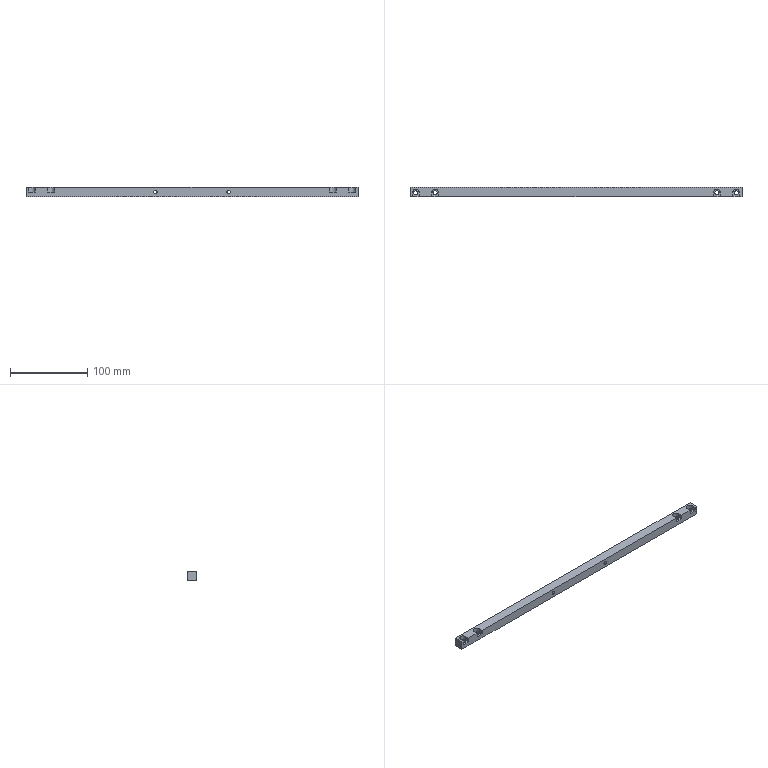Part | SolidWorks | features HoleWzd 2, Extrusion 1, ICE 1 | 1 solid | 40 faces | box 430 x 12 x 12 mm | volume 58809 mm3 | cylinder 20 | plane 20 | commonest cylinder face diameters 5.5 x8 4.5 x4 8 x4 9 x4
STEP:
#1=CARTESIAN_POINT('',(-47.5,1.4,-4.));
#2=VERTEX_POINT('',#1);
#3=CARTESIAN_POINT('',(-47.5,1.4,4.));
#4=VERTEX_POINT('',#3);
#5=CARTESIAN_POINT('',(-47.5,1.4,0.));
#6=DIRECTION('',(0.,1.,0.));
#7=DIRECTION('',(0.,0.,1.));
#8=AXIS2_PLACEMENT_3D('',#5,#6,#7);
#9=CIRCLE('',#8,4.);
#10=EDGE_CURVE('',#2,#4,#9,.T.);
#11=ORIENTED_EDGE('',*,*,#10,.F.);
#12=CARTESIAN_POINT('',(-47.5,6.,-4.));
#13=VERTEX_POINT('',#12);
#14=CARTESIAN_POINT('',(-47.5,6.,-4.));
#15=DIRECTION('',(0.,1.,0.));
#16=VECTOR('',#15,1000.);
#17=LINE('',#14,#16);
#18=EDGE_CURVE('',#2,#13,#17,.T.);
#19=ORIENTED_EDGE('',*,*,#18,.T.);
#20=CARTESIAN_POINT('',(-47.5,6.,4.));
#21=VERTEX_POINT('',#20);
#22=CARTESIAN_POINT('',(-47.5,6.,0.));
#23=DIRECTION('',(0.,1.,0.));
#24=DIRECTION('',(0.,0.,1.));
#25=AXIS2_PLACEMENT_3D('',#22,#23,#24);
#26=CIRCLE('',#25,4.);
#27=EDGE_CURVE('',#13,#21,#26,.T.);
#28=ORIENTED_EDGE('',*,*,#27,.T.);
#29=CARTESIAN_POINT('',(-47.5,6.,4.));
#30=DIRECTION('',(0.,1.,0.));
#31=VECTOR('',#30,1000.);
#32=LINE('',#29,#31);
#33=EDGE_CURVE('',#4,#21,#32,.T.);
#34=ORIENTED_EDGE('',*,*,#33,.F.);
#35=EDGE_LOOP('',(#11,#19,#28,#34));
#36=FACE_OUTER_BOUND('',#35,.T.);
#37=CARTESIAN_POINT('',(-47.5,6.,0.));
#38=DIRECTION('',(0.,1.,0.));
#39=DIRECTION('',(0.,0.,1.));
#40=AXIS2_PLACEMENT_3D('',#37,#38,#39);
#41=CYLINDRICAL_SURFACE('',#40,4.);
#42=ADVANCED_FACE('',(#36),#41,.F.);
#43=CARTESIAN_POINT('',(-47.5,-6.,-2.25));
#44=VERTEX_POINT('',#43);
#45=CARTESIAN_POINT('',(-47.5,-6.,2.25));
#46=VERTEX_POINT('',#45);
#47=CARTESIAN_POINT('',(-47.5,-6.,0.));
#48=DIRECTION('',(0.,1.,0.));
#49=DIRECTION('',(0.,0.,1.));
#50=AXIS2_PLACEMENT_3D('',#47,#48,#49);
#51=CIRCLE('',#50,2.25);
#52=EDGE_CURVE('',#44,#46,#51,.T.);
#53=ORIENTED_EDGE('',*,*,#52,.F.);
#54=CARTESIAN_POINT('',(-47.5,1.4,-2.25));
#55=VERTEX_POINT('',#54);
#56=CARTESIAN_POINT('',(-47.5,6.,-2.25));
#57=DIRECTION('',(0.,1.,0.));
#58=VECTOR('',#57,1000.);
#59=LINE('',#56,#58);
#60=EDGE_CURVE('',#44,#55,#59,.T.);
#61=ORIENTED_EDGE('',*,*,#60,.T.);
#62=CARTESIAN_POINT('',(-47.5,1.4,2.25));
#63=VERTEX_POINT('',#62);
#64=CARTESIAN_POINT('',(-47.5,1.4,0.));
#65=DIRECTION('',(0.,1.,0.));
#66=DIRECTION('',(0.,0.,1.));
#67=AXIS2_PLACEMENT_3D('',#64,#65,#66);
#68=CIRCLE('',#67,2.25);
#69=EDGE_CURVE('',#55,#63,#68,.T.);
#70=ORIENTED_EDGE('',*,*,#69,.T.);
#71=CARTESIAN_POINT('',(-47.5,6.,2.25));
#72=DIRECTION('',(0.,1.,0.));
#73=VECTOR('',#72,1000.);
#74=LINE('',#71,#73);
#75=EDGE_CURVE('',#46,#63,#74,.T.);
#76=ORIENTED_EDGE('',*,*,#75,.F.);
#77=EDGE_LOOP('',(#53,#61,#70,#76));
#78=FACE_OUTER_BOUND('',#77,.T.);
#79=CARTESIAN_POINT('',(-47.5,6.,0.));
#80=DIRECTION('',(0.,1.,0.));
#81=DIRECTION('',(0.,0.,1.));
#82=AXIS2_PLACEMENT_3D('',#79,#80,#81);
#83=CYLINDRICAL_SURFACE('',#82,2.25);
#84=ADVANCED_FACE('',(#78),#83,.F.);
#85=CARTESIAN_POINT('',(47.5,1.4,-4.));
#86=VERTEX_POINT('',#85);
#87=CARTESIAN_POINT('',(47.5,1.4,4.));
#88=VERTEX_POINT('',#87);
#89=CARTESIAN_POINT('',(47.5,1.4,0.));
#90=DIRECTION('',(0.,1.,0.));
#91=DIRECTION('',(0.,0.,1.));
#92=AXIS2_PLACEMENT_3D('',#89,#90,#91);
#93=CIRCLE('',#92,4.);
#94=EDGE_CURVE('',#86,#88,#93,.T.);
#95=ORIENTED_EDGE('',*,*,#94,.F.);
#96=CARTESIAN_POINT('',(47.5,6.,-4.));
#97=VERTEX_POINT('',#96);
#98=CARTESIAN_POINT('',(47.5,6.,-4.));
#99=DIRECTION('',(0.,1.,0.));
#100=VECTOR('',#99,1000.);
#101=LINE('',#98,#100);
#102=EDGE_CURVE('',#86,#97,#101,.T.);
#103=ORIENTED_EDGE('',*,*,#102,.T.);
#104=CARTESIAN_POINT('',(47.5,6.,4.));
#105=VERTEX_POINT('',#104);
#106=CARTESIAN_POINT('',(47.5,6.,0.));
#107=DIRECTION('',(0.,1.,0.));
#108=DIRECTION('',(0.,0.,1.));
#109=AXIS2_PLACEMENT_3D('',#106,#107,#108);
#110=CIRCLE('',#109,4.);
#111=EDGE_CURVE('',#97,#105,#110,.T.);
#112=ORIENTED_EDGE('',*,*,#111,.T.);
#113=CARTESIAN_POINT('',(47.5,6.,4.));
#114=DIRECTION('',(0.,1.,0.));
#115=VECTOR('',#114,1000.);
#116=LINE('',#113,#115);
#117=EDGE_CURVE('',#88,#105,#116,.T.);
#118=ORIENTED_EDGE('',*,*,#117,.F.);
#119=EDGE_LOOP('',(#95,#103,#112,#118));
#120=FACE_OUTER_BOUND('',#119,.T.);
#121=CARTESIAN_POINT('',(47.5,6.,0.));
#122=DIRECTION('',(0.,1.,0.));
#123=DIRECTION('',(0.,0.,1.));
#124=AXIS2_PLACEMENT_3D('',#121,#122,#123);
#125=CYLINDRICAL_SURFACE('',#124,4.);
#126=ADVANCED_FACE('',(#120),#125,.F.);
#127=CARTESIAN_POINT('',(47.5,-6.,-2.25));
#128=VERTEX_POINT('',#127);
#129=CARTESIAN_POINT('',(47.5,-6.,2.25));
#130=VERTEX_POINT('',#129);
#131=CARTESIAN_POINT('',(47.5,-6.,0.));
#132=DIRECTION('',(0.,1.,0.));
#133=DIRECTION('',(0.,0.,1.));
#134=AXIS2_PLACEMENT_3D('',#131,#132,#133);
#135=CIRCLE('',#134,2.25);
#136=EDGE_CURVE('',#128,#130,#135,.T.);
#137=ORIENTED_EDGE('',*,*,#136,.F.);
#138=CARTESIAN_POINT('',(47.5,1.4,-2.25));
#139=VERTEX_POINT('',#138);
#140=CARTESIAN_POINT('',(47.5,6.,-2.25));
#141=DIRECTION('',(0.,1.,0.));
#142=VECTOR('',#141,1000.);
#143=LINE('',#140,#142);
#144=EDGE_CURVE('',#128,#139,#143,.T.);
#145=ORIENTED_EDGE('',*,*,#144,.T.);
#146=CARTESIAN_POINT('',(47.5,1.4,2.25));
#147=VERTEX_POINT('',#146);
#148=CARTESIAN_POINT('',(47.5,1.4,0.));
#149=DIRECTION('',(0.,1.,0.));
#150=DIRECTION('',(0.,0.,1.));
#151=AXIS2_PLACEMENT_3D('',#148,#149,#150);
#152=CIRCLE('',#151,2.25);
#153=EDGE_CURVE('',#139,#147,#152,.T.);
#154=ORIENTED_EDGE('',*,*,#153,.T.);
#155=CARTESIAN_POINT('',(47.5,6.,2.25));
#156=DIRECTION('',(0.,1.,0.));
#157=VECTOR('',#156,1000.);
#158=LINE('',#155,#157);
#159=EDGE_CURVE('',#130,#147,#158,.T.);
#160=ORIENTED_EDGE('',*,*,#159,.F.);
#161=EDGE_LOOP('',(#137,#145,#154,#160));
#162=FACE_OUTER_BOUND('',#161,.T.);
#163=CARTESIAN_POINT('',(47.5,6.,0.));
#164=DIRECTION('',(0.,1.,0.));
#165=DIRECTION('',(0.,0.,1.));
#166=AXIS2_PLACEMENT_3D('',#163,#164,#165);
#167=CYLINDRICAL_SURFACE('',#166,2.25);
#168=ADVANCED_FACE('',(#162),#167,.F.);
#169=CARTESIAN_POINT('',(-210.25,-1.,-6.));
#170=VERTEX_POINT('',#169);
#171=CARTESIAN_POINT('',(-204.75,-1.,-6.));
#172=VERTEX_POINT('',#171);
#173=CARTESIAN_POINT('',(-207.5,-1.,-6.));
#174=DIRECTION('',(0.,0.,1.));
#175=DIRECTION('',(1.,0.,0.));
#176=AXIS2_PLACEMENT_3D('',#173,#174,#175);
#177=CIRCLE('',#176,2.75);
#178=EDGE_CURVE('',#170,#172,#177,.T.);
#179=ORIENTED_EDGE('',*,*,#178,.F.);
#180=CARTESIAN_POINT('',(-210.25,-1.,0.));
#181=VERTEX_POINT('',#180);
#182=CARTESIAN_POINT('',(-210.25,-1.,6.));
#183=DIRECTION('',(0.,0.,1.));
#184=VECTOR('',#183,1000.);
#185=LINE('',#182,#184);
#186=EDGE_CURVE('',#170,#181,#185,.T.);
#187=ORIENTED_EDGE('',*,*,#186,.T.);
#188=CARTESIAN_POINT('',(-204.75,-1.,0.));
#189=VERTEX_POINT('',#188);
#190=CARTESIAN_POINT('',(-207.5,-1.,0.));
#191=DIRECTION('',(0.,0.,-1.));
#192=DIRECTION('',(1.,0.,0.));
#193=AXIS2_PLACEMENT_3D('',#190,#191,#192);
#194=CIRCLE('',#193,2.75);
#195=EDGE_CURVE('',#189,#181,#194,.T.);
#196=ORIENTED_EDGE('',*,*,#195,.F.);
#197=CARTESIAN_POINT('',(-204.75,-1.,6.));
#198=DIRECTION('',(0.,0.,1.));
#199=VECTOR('',#198,1000.);
#200=LINE('',#197,#199);
#201=EDGE_CURVE('',#172,#189,#200,.T.);
#202=ORIENTED_EDGE('',*,*,#201,.F.);
#203=EDGE_LOOP('',(#179,#187,#196,#202));
#204=FACE_OUTER_BOUND('',#203,.T.);
#205=CARTESIAN_POINT('',(-207.5,-1.,6.));
#206=DIRECTION('',(0.,0.,1.));
#207=DIRECTION('',(1.,0.,0.));
#208=AXIS2_PLACEMENT_3D('',#205,#206,#207);
#209=CYLINDRICAL_SURFACE('',#208,2.75);
#210=ADVANCED_FACE('',(#204),#209,.F.);
#211=CARTESIAN_POINT('',(-185.25,-1.,-6.));
#212=VERTEX_POINT('',#211);
#213=CARTESIAN_POINT('',(-179.75,-1.,-6.));
#214=VERTEX_POINT('',#213);
#215=CARTESIAN_POINT('',(-182.5,-1.,-6.));
#216=DIRECTION('',(0.,0.,1.));
#217=DIRECTION('',(1.,0.,0.));
#218=AXIS2_PLACEMENT_3D('',#215,#216,#217);
#219=CIRCLE('',#218,2.75);
#220=EDGE_CURVE('',#212,#214,#219,.T.);
#221=ORIENTED_EDGE('',*,*,#220,.F.);
#222=CARTESIAN_POINT('',(-185.25,-1.,0.));
#223=VERTEX_POINT('',#222);
#224=CARTESIAN_POINT('',(-185.25,-1.,6.));
#225=DIRECTION('',(0.,0.,1.));
#226=VECTOR('',#225,1000.);
#227=LINE('',#224,#226);
#228=EDGE_CURVE('',#212,#223,#227,.T.);
#229=ORIENTED_EDGE('',*,*,#228,.T.);
#230=CARTESIAN_POINT('',(-179.75,-1.,0.));
#231=VERTEX_POINT('',#230);
#232=CARTESIAN_POINT('',(-182.5,-1.,0.));
#233=DIRECTION('',(0.,0.,-1.));
#234=DIRECTION('',(1.,0.,0.));
#235=AXIS2_PLACEMENT_3D('',#232,#233,#234);
#236=CIRCLE('',#235,2.75);
#237=EDGE_CURVE('',#231,#223,#236,.T.);
#238=ORIENTED_EDGE('',*,*,#237,.F.);
#239=CARTESIAN_POINT('',(-179.75,-1.,6.));
#240=DIRECTION('',(0.,0.,1.));
#241=VECTOR('',#240,1000.);
#242=LINE('',#239,#241);
#243=EDGE_CURVE('',#214,#231,#242,.T.);
#244=ORIENTED_EDGE('',*,*,#243,.F.);
#245=EDGE_LOOP('',(#221,#229,#238,#244));
#246=FACE_OUTER_BOUND('',#245,.T.);
#247=CARTESIAN_POINT('',(-182.5,-1.,6.));
#248=DIRECTION('',(0.,0.,1.));
#249=DIRECTION('',(1.,0.,0.));
#250=AXIS2_PLACEMENT_3D('',#247,#248,#249);
#251=CYLINDRICAL_SURFACE('',#250,2.75);
#252=ADVANCED_FACE('',(#246),#251,.F.);
#253=CARTESIAN_POINT('',(179.75,-1.,-6.));
#254=VERTEX_POINT('',#253);
#255=CARTESIAN_POINT('',(185.25,-1.,-6.));
#256=VERTEX_POINT('',#255);
#257=CARTESIAN_POINT('',(182.5,-1.,-6.));
#258=DIRECTION('',(0.,0.,1.));
#259=DIRECTION('',(1.,0.,0.));
#260=AXIS2_PLACEMENT_3D('',#257,#258,#259);
#261=CIRCLE('',#260,2.75);
#262=EDGE_CURVE('',#254,#256,#261,.T.);
#263=ORIENTED_EDGE('',*,*,#262,.F.);
#264=CARTESIAN_POINT('',(179.75,-1.,0.));
#265=VERTEX_POINT('',#264);
#266=CARTESIAN_POINT('',(179.75,-1.,6.));
#267=DIRECTION('',(0.,0.,1.));
#268=VECTOR('',#267,1000.);
#269=LINE('',#266,#268);
#270=EDGE_CURVE('',#254,#265,#269,.T.);
#271=ORIENTED_EDGE('',*,*,#270,.T.);
#272=CARTESIAN_POINT('',(185.25,-1.,0.));
#273=VERTEX_POINT('',#272);
#274=CARTESIAN_POINT('',(182.5,-1.,0.));
#275=DIRECTION('',(0.,0.,-1.));
#276=DIRECTION('',(1.,0.,0.));
#277=AXIS2_PLACEMENT_3D('',#274,#275,#276);
#278=CIRCLE('',#277,2.75);
#279=EDGE_CURVE('',#273,#265,#278,.T.);
#280=ORIENTED_EDGE('',*,*,#279,.F.);
#281=CARTESIAN_POINT('',(185.25,-1.,6.));
#282=DIRECTION('',(0.,0.,1.));
#283=VECTOR('',#282,1000.);
#284=LINE('',#281,#283);
#285=EDGE_CURVE('',#256,#273,#284,.T.);
#286=ORIENTED_EDGE('',*,*,#285,.F.);
#287=EDGE_LOOP('',(#263,#271,#280,#286));
#288=FACE_OUTER_BOUND('',#287,.T.);
#289=CARTESIAN_POINT('',(182.5,-1.,6.));
#290=DIRECTION('',(0.,0.,1.));
#291=DIRECTION('',(1.,0.,0.));
#292=AXIS2_PLACEMENT_3D('',#289,#290,#291);
#293=CYLINDRICAL_SURFACE('',#292,2.75);
#294=ADVANCED_FACE('',(#288),#293,.F.);
#295=CARTESIAN_POINT('',(204.75,-1.,-6.));
#296=VERTEX_POINT('',#295);
#297=CARTESIAN_POINT('',(210.25,-1.,-6.));
#298=VERTEX_POINT('',#297);
#299=CARTESIAN_POINT('',(207.5,-1.,-6.));
#300=DIRECTION('',(0.,0.,1.));
#301=DIRECTION('',(1.,0.,0.));
#302=AXIS2_PLACEMENT_3D('',#299,#300,#301);
#303=CIRCLE('',#302,2.75);
#304=EDGE_CURVE('',#296,#298,#303,.T.);
#305=ORIENTED_EDGE('',*,*,#304,.F.);
#306=CARTESIAN_POINT('',(204.75,-1.,0.));
#307=VERTEX_POINT('',#306);
#308=CARTESIAN_POINT('',(204.75,-1.,6.));
#309=DIRECTION('',(0.,0.,1.));
#310=VECTOR('',#309,1000.);
#311=LINE('',#308,#310);
#312=EDGE_CURVE('',#296,#307,#311,.T.);
#313=ORIENTED_EDGE('',*,*,#312,.T.);
#314=CARTESIAN_POINT('',(210.25,-1.,0.));
#315=VERTEX_POINT('',#314);
#316=CARTESIAN_POINT('',(207.5,-1.,0.));
#317=DIRECTION('',(0.,0.,-1.));
#318=DIRECTION('',(1.,0.,0.));
#319=AXIS2_PLACEMENT_3D('',#316,#317,#318);
#320=CIRCLE('',#319,2.75);
#321=EDGE_CURVE('',#315,#307,#320,.T.);
#322=ORIENTED_EDGE('',*,*,#321,.F.);
#323=CARTESIAN_POINT('',(210.25,-1.,6.));
#324=DIRECTION('',(0.,0.,1.));
#325=VECTOR('',#324,1000.);
#326=LINE('',#323,#325);
#327=EDGE_CURVE('',#298,#315,#326,.T.);
#328=ORIENTED_EDGE('',*,*,#327,.F.);
#329=EDGE_LOOP('',(#305,#313,#322,#328));
#330=FACE_OUTER_BOUND('',#329,.T.);
#331=CARTESIAN_POINT('',(207.5,-1.,6.));
#332=DIRECTION('',(0.,0.,1.));
#333=DIRECTION('',(1.,0.,0.));
#334=AXIS2_PLACEMENT_3D('',#331,#332,#333);
#335=CYLINDRICAL_SURFACE('',#334,2.75);
#336=ADVANCED_FACE('',(#330),#335,.F.);
#337=ORIENTED_EDGE('',*,*,#312,.F.);
#338=CARTESIAN_POINT('',(207.5,-1.,-6.));
#339=DIRECTION('',(0.,0.,1.));
#340=DIRECTION('',(1.,0.,0.));
#341=AXIS2_PLACEMENT_3D('',#338,#339,#340);
#342=CIRCLE('',#341,2.75);
#343=EDGE_CURVE('',#298,#296,#342,.T.);
#344=ORIENTED_EDGE('',*,*,#343,.F.);
#345=ORIENTED_EDGE('',*,*,#327,.T.);
#346=CARTESIAN_POINT('',(207.5,-1.,0.));
#347=DIRECTION('',(0.,0.,-1.));
#348=DIRECTION('',(1.,0.,0.));
#349=AXIS2_PLACEMENT_3D('',#346,#347,#348);
#350=CIRCLE('',#349,2.75);
#351=EDGE_CURVE('',#307,#315,#350,.T.);
#352=ORIENTED_EDGE('',*,*,#351,.F.);
#353=EDGE_LOOP('',(#337,#344,#345,#352));
#354=FACE_OUTER_BOUND('',#353,.T.);
#355=CARTESIAN_POINT('',(207.5,-1.,6.));
#356=DIRECTION('',(0.,0.,1.));
#357=DIRECTION('',(1.,0.,0.));
#358=AXIS2_PLACEMENT_3D('',#355,#356,#357);
#359=CYLINDRICAL_SURFACE('',#358,2.75);
#360=ADVANCED_FACE('',(#354),#359,.F.);
#361=ORIENTED_EDGE('',*,*,#270,.F.);
#362=CARTESIAN_POINT('',(182.5,-1.,-6.));
#363=DIRECTION('',(0.,0.,1.));
#364=DIRECTION('',(1.,0.,0.));
#365=AXIS2_PLACEMENT_3D('',#362,#363,#364);
#366=CIRCLE('',#365,2.75);
#367=EDGE_CURVE('',#256,#254,#366,.T.);
#368=ORIENTED_EDGE('',*,*,#367,.F.);
#369=ORIENTED_EDGE('',*,*,#285,.T.);
#370=CARTESIAN_POINT('',(182.5,-1.,0.));
#371=DIRECTION('',(0.,0.,-1.));
#372=DIRECTION('',(1.,0.,0.));
#373=AXIS2_PLACEMENT_3D('',#370,#371,#372);
#374=CIRCLE('',#373,2.75);
#375=EDGE_CURVE('',#265,#273,#374,.T.);
#376=ORIENTED_EDGE('',*,*,#375,.F.);
#377=EDGE_LOOP('',(#361,#368,#369,#376));
#378=FACE_OUTER_BOUND('',#377,.T.);
#379=CARTESIAN_POINT('',(182.5,-1.,6.));
#380=DIRECTION('',(0.,0.,1.));
#381=DIRECTION('',(1.,0.,0.));
#382=AXIS2_PLACEMENT_3D('',#379,#380,#381);
#383=CYLINDRICAL_SURFACE('',#382,2.75);
#384=ADVANCED_FACE('',(#378),#383,.F.);
#385=ORIENTED_EDGE('',*,*,#228,.F.);
#386=CARTESIAN_POINT('',(-182.5,-1.,-6.));
#387=DIRECTION('',(0.,0.,1.));
#388=DIRECTION('',(1.,0.,0.));
#389=AXIS2_PLACEMENT_3D('',#386,#387,#388);
#390=CIRCLE('',#389,2.75);
#391=EDGE_CURVE('',#214,#212,#390,.T.);
#392=ORIENTED_EDGE('',*,*,#391,.F.);
#393=ORIENTED_EDGE('',*,*,#243,.T.);
#394=CARTESIAN_POINT('',(-182.5,-1.,0.));
#395=DIRECTION('',(0.,0.,-1.));
#396=DIRECTION('',(1.,0.,0.));
#397=AXIS2_PLACEMENT_3D('',#394,#395,#396);
#398=CIRCLE('',#397,2.75);
#399=EDGE_CURVE('',#223,#231,#398,.T.);
#400=ORIENTED_EDGE('',*,*,#399,.F.);
#401=EDGE_LOOP('',(#385,#392,#393,#400));
#402=FACE_OUTER_BOUND('',#401,.T.);
#403=CARTESIAN_POINT('',(-182.5,-1.,6.));
#404=DIRECTION('',(0.,0.,1.));
#405=DIRECTION('',(1.,0.,0.));
#406=AXIS2_PLACEMENT_3D('',#403,#404,#405);
#407=CYLINDRICAL_SURFACE('',#406,2.75);
#408=ADVANCED_FACE('',(#402),#407,.F.);
#409=ORIENTED_EDGE('',*,*,#186,.F.);
#410=CARTESIAN_POINT('',(-207.5,-1.,-6.));
#411=DIRECTION('',(0.,0.,1.));
#412=DIRECTION('',(1.,0.,0.));
#413=AXIS2_PLACEMENT_3D('',#410,#411,#412);
#414=CIRCLE('',#413,2.75);
#415=EDGE_CURVE('',#172,#170,#414,.T.);
#416=ORIENTED_EDGE('',*,*,#415,.F.);
#417=ORIENTED_EDGE('',*,*,#201,.T.);
#418=CARTESIAN_POINT('',(-207.5,-1.,0.));
#419=DIRECTION('',(0.,0.,-1.));
#420=DIRECTION('',(1.,0.,0.));
#421=AXIS2_PLACEMENT_3D('',#418,#419,#420);
#422=CIRCLE('',#421,2.75);
#423=EDGE_CURVE('',#181,#189,#422,.T.);
#424=ORIENTED_EDGE('',*,*,#423,.F.);
#425=EDGE_LOOP('',(#409,#416,#417,#424));
#426=FACE_OUTER_BOUND('',#425,.T.);
#427=CARTESIAN_POINT('',(-207.5,-1.,6.));
#428=DIRECTION('',(0.,0.,1.));
#429=DIRECTION('',(1.,0.,0.));
#430=AXIS2_PLACEMENT_3D('',#427,#428,#429);
#431=CYLINDRICAL_SURFACE('',#430,2.75);
#432=ADVANCED_FACE('',(#426),#431,.F.);
#433=CARTESIAN_POINT('',(215.,-6.,-6.));
#434=VERTEX_POINT('',#433);
#435=CARTESIAN_POINT('',(215.,6.,-6.));
#436=VERTEX_POINT('',#435);
#437=CARTESIAN_POINT('',(215.,6.,-6.));
#438=DIRECTION('',(0.,1.,0.));
#439=VECTOR('',#438,1000.);
#440=LINE('',#437,#439);
#441=EDGE_CURVE('',#434,#436,#440,.T.);
#442=ORIENTED_EDGE('',*,*,#441,.T.);
#443=CARTESIAN_POINT('',(215.,6.,6.));
#444=VERTEX_POINT('',#443);
#445=CARTESIAN_POINT('',(215.,6.,6.));
#446=DIRECTION('',(0.,0.,-1.));
#447=VECTOR('',#446,1000.);
#448=LINE('',#445,#447);
#449=EDGE_CURVE('',#444,#436,#448,.T.);
#450=ORIENTED_EDGE('',*,*,#449,.F.);
#451=CARTESIAN_POINT('',(215.,-6.,6.));
#452=VERTEX_POINT('',#451);
#453=CARTESIAN_POINT('',(215.,6.,6.));
#454=DIRECTION('',(0.,1.,0.));
#455=VECTOR('',#454,1000.);
#456=LINE('',#453,#455);
#457=EDGE_CURVE('',#452,#444,#456,.T.);
#458=ORIENTED_EDGE('',*,*,#457,.F.);
#459=CARTESIAN_POINT('',(215.,-6.,6.));
#460=DIRECTION('',(0.,0.,-1.));
#461=VECTOR('',#460,1000.);
#462=LINE('',#459,#461);
#463=EDGE_CURVE('',#452,#434,#462,.T.);
#464=ORIENTED_EDGE('',*,*,#463,.T.);
#465=EDGE_LOOP('',(#442,#450,#458,#464));
#466=FACE_OUTER_BOUND('',#465,.T.);
#467=CARTESIAN_POINT('',(215.,6.,6.));
#468=DIRECTION('',(-1.,0.,0.));
#469=DIRECTION('',(0.,0.,1.));
#470=AXIS2_PLACEMENT_3D('',#467,#468,#469);
#471=PLANE('',#470);
#472=ADVANCED_FACE('',(#466),#471,.F.);
#473=CARTESIAN_POINT('',(-47.5,6.,0.));
#474=DIRECTION('',(0.,1.,0.));
#475=DIRECTION('',(0.,0.,1.));
#476=AXIS2_PLACEMENT_3D('',#473,#474,#475);
#477=CIRCLE('',#476,4.);
#478=EDGE_CURVE('',#21,#13,#477,.T.);
#479=ORIENTED_EDGE('',*,*,#478,.F.);
#480=ORIENTED_EDGE('',*,*,#27,.F.);
#481=EDGE_LOOP('',(#479,#480));
#482=FACE_BOUND('',#481,.T.);
#483=CARTESIAN_POINT('',(47.5,6.,0.));
#484=DIRECTION('',(0.,1.,0.));
#485=DIRECTION('',(0.,0.,1.));
#486=AXIS2_PLACEMENT_3D('',#483,#484,#485);
#487=CIRCLE('',#486,4.);
#488=EDGE_CURVE('',#105,#97,#487,.T.);
#489=ORIENTED_EDGE('',*,*,#488,.F.);
#490=ORIENTED_EDGE('',*,*,#111,.F.);
#491=EDGE_LOOP('',(#489,#490));
#492=FACE_BOUND('',#491,.T.);
#493=CARTESIAN_POINT('',(-215.,6.,-6.));
#494=VERTEX_POINT('',#493);
#495=CARTESIAN_POINT('',(-215.,6.,-6.));
#496=DIRECTION('',(-1.,0.,0.));
#497=VECTOR('',#496,1000.);
#498=LINE('',#495,#497);
#499=EDGE_CURVE('',#436,#494,#498,.T.);
#500=ORIENTED_EDGE('',*,*,#499,.T.);
#501=CARTESIAN_POINT('',(-215.,6.,6.));
#502=VERTEX_POINT('',#501);
#503=CARTESIAN_POINT('',(-215.,6.,6.));
#504=DIRECTION('',(0.,0.,-1.));
#505=VECTOR('',#504,1000.);
#506=LINE('',#503,#505);
#507=EDGE_CURVE('',#502,#494,#506,.T.);
#508=ORIENTED_EDGE('',*,*,#507,.F.);
#509=CARTESIAN_POINT('',(-215.,6.,6.));
#510=DIRECTION('',(-1.,0.,0.));
#511=VECTOR('',#510,1000.);
#512=LINE('',#509,#511);
#513=EDGE_CURVE('',#444,#502,#512,.T.);
#514=ORIENTED_EDGE('',*,*,#513,.F.);
#515=ORIENTED_EDGE('',*,*,#449,.T.);
#516=EDGE_LOOP('',(#500,#508,#514,#515));
#517=FACE_OUTER_BOUND('',#516,.T.);
#518=CARTESIAN_POINT('',(-215.,6.,6.));
#519=DIRECTION('',(0.,-1.,0.));
#520=DIRECTION('',(0.,0.,-1.));
#521=AXIS2_PLACEMENT_3D('',#518,#519,#520);
#522=PLANE('',#521);
#523=ADVANCED_FACE('',(#482,#492,#517),#522,.F.);
#524=CARTESIAN_POINT('',(-215.,-6.,-6.));
#525=VERTEX_POINT('',#524);
#526=CARTESIAN_POINT('',(-215.,6.,-6.));
#527=DIRECTION('',(0.,-1.,0.));
#528=VECTOR('',#527,1000.);
#529=LINE('',#526,#528);
#530=EDGE_CURVE('',#494,#525,#529,.T.);
#531=ORIENTED_EDGE('',*,*,#530,.T.);
#532=CARTESIAN_POINT('',(-215.,-6.,6.));
#533=VERTEX_POINT('',#532);
#534=CARTESIAN_POINT('',(-215.,-6.,6.));
#535=DIRECTION('',(0.,0.,-1.));
#536=VECTOR('',#535,1000.);
#537=LINE('',#534,#536);
#538=EDGE_CURVE('',#533,#525,#537,.T.);
#539=ORIENTED_EDGE('',*,*,#538,.F.);
#540=CARTESIAN_POINT('',(-215.,6.,6.));
#541=DIRECTION('',(0.,-1.,0.));
#542=VECTOR('',#541,1000.);
#543=LINE('',#540,#542);
#544=EDGE_CURVE('',#502,#533,#543,.T.);
#545=ORIENTED_EDGE('',*,*,#544,.F.);
#546=ORIENTED_EDGE('',*,*,#507,.T.);
#547=EDGE_LOOP('',(#531,#539,#545,#546));
#548=FACE_OUTER_BOUND('',#547,.T.);
#549=CARTESIAN_POINT('',(-215.,6.,6.));
#550=DIRECTION('',(1.,0.,0.));
#551=DIRECTION('',(0.,0.,-1.));
#552=AXIS2_PLACEMENT_3D('',#549,#550,#551);
#553=PLANE('',#552);
#554=ADVANCED_FACE('',(#548),#553,.F.);
#555=CARTESIAN_POINT('',(212.,-6.,6.));
#556=VERTEX_POINT('',#555);
#557=CARTESIAN_POINT('',(-215.,-6.,6.));
#558=DIRECTION('',(1.,0.,0.));
#559=VECTOR('',#558,1000.);
#560=LINE('',#557,#559);
#561=EDGE_CURVE('',#556,#452,#560,.T.);
#562=ORIENTED_EDGE('',*,*,#561,.F.);
#563=CARTESIAN_POINT('',(212.,-6.,0.));
#564=VERTEX_POINT('',#563);
#565=CARTESIAN_POINT('',(212.,-6.,6.));
#566=DIRECTION('',(0.,0.,-1.));
#567=VECTOR('',#566,1000.);
#568=LINE('',#565,#567);
#569=EDGE_CURVE('',#556,#564,#568,.T.);
#570=ORIENTED_EDGE('',*,*,#569,.T.);
#571=CARTESIAN_POINT('',(203.,-6.,0.));
#572=VERTEX_POINT('',#571);
#573=CARTESIAN_POINT('',(-215.,-6.,0.));
#574=DIRECTION('',(1.,0.,0.));
#575=VECTOR('',#574,1000.);
#576=LINE('',#573,#575);
#577=EDGE_CURVE('',#572,#564,#576,.T.);
#578=ORIENTED_EDGE('',*,*,#577,.F.);
#579=CARTESIAN_POINT('',(203.,-6.,6.));
#580=VERTEX_POINT('',#579);
#581=CARTESIAN_POINT('',(203.,-6.,6.));
#582=DIRECTION('',(0.,0.,1.));
#583=VECTOR('',#582,1000.);
#584=LINE('',#581,#583);
#585=EDGE_CURVE('',#572,#580,#584,.T.);
#586=ORIENTED_EDGE('',*,*,#585,.T.);
#587=CARTESIAN_POINT('',(187.,-6.,6.));
#588=VERTEX_POINT('',#587);
#589=CARTESIAN_POINT('',(-215.,-6.,6.));
#590=DIRECTION('',(1.,0.,0.));
#591=VECTOR('',#590,1000.);
#592=LINE('',#589,#591);
#593=EDGE_CURVE('',#588,#580,#592,.T.);
#594=ORIENTED_EDGE('',*,*,#593,.F.);
#595=CARTESIAN_POINT('',(187.,-6.,0.));
#596=VERTEX_POINT('',#595);
#597=CARTESIAN_POINT('',(187.,-6.,6.));
#598=DIRECTION('',(0.,0.,-1.));
#599=VECTOR('',#598,1000.);
#600=LINE('',#597,#599);
#601=EDGE_CURVE('',#588,#596,#600,.T.);
#602=ORIENTED_EDGE('',*,*,#601,.T.);
#603=CARTESIAN_POINT('',(178.,-6.,0.));
#604=VERTEX_POINT('',#603);
#605=CARTESIAN_POINT('',(-215.,-6.,0.));
#606=DIRECTION('',(1.,0.,0.));
#607=VECTOR('',#606,1000.);
#608=LINE('',#605,#607);
#609=EDGE_CURVE('',#604,#596,#608,.T.);
#610=ORIENTED_EDGE('',*,*,#609,.F.);
#611=CARTESIAN_POINT('',(178.,-6.,6.));
#612=VERTEX_POINT('',#611);
#613=CARTESIAN_POINT('',(178.,-6.,6.));
#614=DIRECTION('',(0.,0.,1.));
#615=VECTOR('',#614,1000.);
#616=LINE('',#613,#615);
#617=EDGE_CURVE('',#604,#612,#616,.T.);
#618=ORIENTED_EDGE('',*,*,#617,.T.);
#619=CARTESIAN_POINT('',(-178.,-6.,6.));
#620=VERTEX_POINT('',#619);
#621=CARTESIAN_POINT('',(-215.,-6.,6.));
#622=DIRECTION('',(1.,0.,0.));
#623=VECTOR('',#622,1000.);
#624=LINE('',#621,#623);
#625=EDGE_CURVE('',#620,#612,#624,.T.);
#626=ORIENTED_EDGE('',*,*,#625,.F.);
#627=CARTESIAN_POINT('',(-178.,-6.,0.));
#628=VERTEX_POINT('',#627);
#629=CARTESIAN_POINT('',(-178.,-6.,6.));
#630=DIRECTION('',(0.,0.,-1.));
#631=VECTOR('',#630,1000.);
#632=LINE('',#629,#631);
#633=EDGE_CURVE('',#620,#628,#632,.T.);
#634=ORIENTED_EDGE('',*,*,#633,.T.);
#635=CARTESIAN_POINT('',(-187.,-6.,0.));
#636=VERTEX_POINT('',#635);
#637=CARTESIAN_POINT('',(-215.,-6.,0.));
#638=DIRECTION('',(1.,0.,0.));
#639=VECTOR('',#638,1000.);
#640=LINE('',#637,#639);
#641=EDGE_CURVE('',#636,#628,#640,.T.);
#642=ORIENTED_EDGE('',*,*,#641,.F.);
#643=CARTESIAN_POINT('',(-187.,-6.,6.));
#644=VERTEX_POINT('',#643);
#645=CARTESIAN_POINT('',(-187.,-6.,6.));
#646=DIRECTION('',(0.,0.,1.));
#647=VECTOR('',#646,1000.);
#648=LINE('',#645,#647);
#649=EDGE_CURVE('',#636,#644,#648,.T.);
#650=ORIENTED_EDGE('',*,*,#649,.T.);
#651=CARTESIAN_POINT('',(-203.,-6.,6.));
#652=VERTEX_POINT('',#651);
#653=CARTESIAN_POINT('',(-215.,-6.,6.));
#654=DIRECTION('',(1.,0.,0.));
#655=VECTOR('',#654,1000.);
#656=LINE('',#653,#655);
#657=EDGE_CURVE('',#652,#644,#656,.T.);
#658=ORIENTED_EDGE('',*,*,#657,.F.);
#659=CARTESIAN_POINT('',(-203.,-6.,0.));
#660=VERTEX_POINT('',#659);
#661=CARTESIAN_POINT('',(-203.,-6.,6.));
#662=DIRECTION('',(0.,0.,-1.));
#663=VECTOR('',#662,1000.);
#664=LINE('',#661,#663);
#665=EDGE_CURVE('',#652,#660,#664,.T.);
#666=ORIENTED_EDGE('',*,*,#665,.T.);
#667=CARTESIAN_POINT('',(-212.,-6.,0.));
#668=VERTEX_POINT('',#667);
#669=CARTESIAN_POINT('',(-215.,-6.,0.));
#670=DIRECTION('',(1.,0.,0.));
#671=VECTOR('',#670,1000.);
#672=LINE('',#669,#671);
#673=EDGE_CURVE('',#668,#660,#672,.T.);
#674=ORIENTED_EDGE('',*,*,#673,.F.);
#675=CARTESIAN_POINT('',(-212.,-6.,6.));
#676=VERTEX_POINT('',#675);
#677=CARTESIAN_POINT('',(-212.,-6.,6.));
#678=DIRECTION('',(0.,0.,1.));
#679=VECTOR('',#678,1000.);
#680=LINE('',#677,#679);
#681=EDGE_CURVE('',#668,#676,#680,.T.);
#682=ORIENTED_EDGE('',*,*,#681,.T.);
#683=CARTESIAN_POINT('',(-215.,-6.,6.));
#684=DIRECTION('',(1.,0.,0.));
#685=VECTOR('',#684,1000.);
#686=LINE('',#683,#685);
#687=EDGE_CURVE('',#533,#676,#686,.T.);
#688=ORIENTED_EDGE('',*,*,#687,.F.);
#689=ORIENTED_EDGE('',*,*,#538,.T.);
#690=CARTESIAN_POINT('',(-215.,-6.,-6.));
#691=DIRECTION('',(1.,0.,0.));
#692=VECTOR('',#691,1000.);
#693=LINE('',#690,#692);
#694=EDGE_CURVE('',#525,#434,#693,.T.);
#695=ORIENTED_EDGE('',*,*,#694,.T.);
#696=ORIENTED_EDGE('',*,*,#463,.F.);
#697=EDGE_LOOP('',(#562,#570,#578,#586,#594,#602,#610,#618,#626,#634,#642,#650,#658,#666,#674,#682,#688,#689,#695,#696));
#698=FACE_OUTER_BOUND('',#697,.T.);
#699=CARTESIAN_POINT('',(-47.5,-6.,0.));
#700=DIRECTION('',(0.,1.,0.));
#701=DIRECTION('',(0.,0.,1.));
#702=AXIS2_PLACEMENT_3D('',#699,#700,#701);
#703=CIRCLE('',#702,2.25);
#704=EDGE_CURVE('',#46,#44,#703,.T.);
#705=ORIENTED_EDGE('',*,*,#704,.T.);
#706=ORIENTED_EDGE('',*,*,#52,.T.);
#707=EDGE_LOOP('',(#705,#706));
#708=FACE_BOUND('',#707,.T.);
#709=CARTESIAN_POINT('',(47.5,-6.,0.));
#710=DIRECTION('',(0.,1.,0.));
#711=DIRECTION('',(0.,0.,1.));
#712=AXIS2_PLACEMENT_3D('',#709,#710,#711);
#713=CIRCLE('',#712,2.25);
#714=EDGE_CURVE('',#130,#128,#713,.T.);
#715=ORIENTED_EDGE('',*,*,#714,.T.);
#716=ORIENTED_EDGE('',*,*,#136,.T.);
#717=EDGE_LOOP('',(#715,#716));
#718=FACE_BOUND('',#717,.T.);
#719=CARTESIAN_POINT('',(-215.,-6.,6.));
#720=DIRECTION('',(0.,1.,0.));
#721=DIRECTION('',(0.,0.,1.));
#722=AXIS2_PLACEMENT_3D('',#719,#720,#721);
#723=PLANE('',#722);
#724=ADVANCED_FACE('',(#698,#708,#718),#723,.F.);
#725=CARTESIAN_POINT('',(212.,-1.,6.));
#726=VERTEX_POINT('',#725);
#727=CARTESIAN_POINT('',(212.,-1.,6.));
#728=DIRECTION('',(0.,1.,0.));
#729=VECTOR('',#728,1000.);
#730=LINE('',#727,#729);
#731=EDGE_CURVE('',#556,#726,#730,.T.);
#732=ORIENTED_EDGE('',*,*,#731,.F.);
#733=ORIENTED_EDGE('',*,*,#561,.T.);
#734=ORIENTED_EDGE('',*,*,#457,.T.);
#735=ORIENTED_EDGE('',*,*,#513,.T.);
#736=ORIENTED_EDGE('',*,*,#544,.T.);
#737=ORIENTED_EDGE('',*,*,#687,.T.);
#738=CARTESIAN_POINT('',(-212.,-1.,6.));
#739=VERTEX_POINT('',#738);
#740=CARTESIAN_POINT('',(-212.,-1.,6.));
#741=DIRECTION('',(0.,-1.,0.));
#742=VECTOR('',#741,1000.);
#743=LINE('',#740,#742);
#744=EDGE_CURVE('',#739,#676,#743,.T.);
#745=ORIENTED_EDGE('',*,*,#744,.F.);
#746=CARTESIAN_POINT('',(-203.,-1.,6.));
#747=VERTEX_POINT('',#746);
#748=CARTESIAN_POINT('',(-207.5,-1.,6.));
#749=DIRECTION('',(0.,0.,1.));
#750=DIRECTION('',(1.,0.,0.));
#751=AXIS2_PLACEMENT_3D('',#748,#749,#750);
#752=CIRCLE('',#751,4.5);
#753=EDGE_CURVE('',#747,#739,#752,.T.);
#754=ORIENTED_EDGE('',*,*,#753,.F.);
#755=CARTESIAN_POINT('',(-203.,-1.,6.));
#756=DIRECTION('',(0.,1.,0.));
#757=VECTOR('',#756,1000.);
#758=LINE('',#755,#757);
#759=EDGE_CURVE('',#652,#747,#758,.T.);
#760=ORIENTED_EDGE('',*,*,#759,.F.);
#761=ORIENTED_EDGE('',*,*,#657,.T.);
#762=CARTESIAN_POINT('',(-187.,-1.,6.));
#763=VERTEX_POINT('',#762);
#764=CARTESIAN_POINT('',(-187.,-1.,6.));
#765=DIRECTION('',(0.,-1.,0.));
#766=VECTOR('',#765,1000.);
#767=LINE('',#764,#766);
#768=EDGE_CURVE('',#763,#644,#767,.T.);
#769=ORIENTED_EDGE('',*,*,#768,.F.);
#770=CARTESIAN_POINT('',(-178.,-1.,6.));
#771=VERTEX_POINT('',#770);
#772=CARTESIAN_POINT('',(-182.5,-1.,6.));
#773=DIRECTION('',(0.,0.,1.));
#774=DIRECTION('',(1.,0.,0.));
#775=AXIS2_PLACEMENT_3D('',#772,#773,#774);
#776=CIRCLE('',#775,4.5);
#777=EDGE_CURVE('',#771,#763,#776,.T.);
#778=ORIENTED_EDGE('',*,*,#777,.F.);
#779=CARTESIAN_POINT('',(-178.,-1.,6.));
#780=DIRECTION('',(0.,1.,0.));
#781=VECTOR('',#780,1000.);
#782=LINE('',#779,#781);
#783=EDGE_CURVE('',#620,#771,#782,.T.);
#784=ORIENTED_EDGE('',*,*,#783,.F.);
#785=ORIENTED_EDGE('',*,*,#625,.T.);
#786=CARTESIAN_POINT('',(178.,-1.,6.));
#787=VERTEX_POINT('',#786);
#788=CARTESIAN_POINT('',(178.,-1.,6.));
#789=DIRECTION('',(0.,-1.,0.));
#790=VECTOR('',#789,1000.);
#791=LINE('',#788,#790);
#792=EDGE_CURVE('',#787,#612,#791,.T.);
#793=ORIENTED_EDGE('',*,*,#792,.F.);
#794=CARTESIAN_POINT('',(187.,-1.,6.));
#795=VERTEX_POINT('',#794);
#796=CARTESIAN_POINT('',(182.5,-1.,6.));
#797=DIRECTION('',(0.,0.,1.));
#798=DIRECTION('',(1.,0.,0.));
#799=AXIS2_PLACEMENT_3D('',#796,#797,#798);
#800=CIRCLE('',#799,4.5);
#801=EDGE_CURVE('',#795,#787,#800,.T.);
#802=ORIENTED_EDGE('',*,*,#801,.F.);
#803=CARTESIAN_POINT('',(187.,-1.,6.));
#804=DIRECTION('',(0.,1.,0.));
#805=VECTOR('',#804,1000.);
#806=LINE('',#803,#805);
#807=EDGE_CURVE('',#588,#795,#806,.T.);
#808=ORIENTED_EDGE('',*,*,#807,.F.);
#809=ORIENTED_EDGE('',*,*,#593,.T.);
#810=CARTESIAN_POINT('',(203.,-1.,6.));
#811=VERTEX_POINT('',#810);
#812=CARTESIAN_POINT('',(203.,-1.,6.));
#813=DIRECTION('',(0.,-1.,0.));
#814=VECTOR('',#813,1000.);
#815=LINE('',#812,#814);
#816=EDGE_CURVE('',#811,#580,#815,.T.);
#817=ORIENTED_EDGE('',*,*,#816,.F.);
#818=CARTESIAN_POINT('',(207.5,-1.,6.));
#819=DIRECTION('',(0.,0.,1.));
#820=DIRECTION('',(1.,0.,0.));
#821=AXIS2_PLACEMENT_3D('',#818,#819,#820);
#822=CIRCLE('',#821,4.5);
#823=EDGE_CURVE('',#726,#811,#822,.T.);
#824=ORIENTED_EDGE('',*,*,#823,.F.);
#825=EDGE_LOOP('',(#732,#733,#734,#735,#736,#737,#745,#754,#760,#761,#769,#778,#784,#785,#793,#802,#808,#809,#817,#824));
#826=FACE_OUTER_BOUND('',#825,.T.);
#827=CARTESIAN_POINT('',(0.,0.,6.));
#828=DIRECTION('',(0.,0.,1.));
#829=DIRECTION('',(1.,0.,0.));
#830=AXIS2_PLACEMENT_3D('',#827,#828,#829);
#831=PLANE('',#830);
#832=ADVANCED_FACE('',(#826),#831,.T.);
#833=ORIENTED_EDGE('',*,*,#415,.T.);
#834=ORIENTED_EDGE('',*,*,#178,.T.);
#835=EDGE_LOOP('',(#833,#834));
#836=FACE_BOUND('',#835,.T.);
#837=ORIENTED_EDGE('',*,*,#391,.T.);
#838=ORIENTED_EDGE('',*,*,#220,.T.);
#839=EDGE_LOOP('',(#837,#838));
#840=FACE_BOUND('',#839,.T.);
#841=ORIENTED_EDGE('',*,*,#367,.T.);
#842=ORIENTED_EDGE('',*,*,#262,.T.);
#843=EDGE_LOOP('',(#841,#842));
#844=FACE_BOUND('',#843,.T.);
#845=ORIENTED_EDGE('',*,*,#343,.T.);
#846=ORIENTED_EDGE('',*,*,#304,.T.);
#847=EDGE_LOOP('',(#845,#846));
#848=FACE_BOUND('',#847,.T.);
#849=ORIENTED_EDGE('',*,*,#441,.F.);
#850=ORIENTED_EDGE('',*,*,#694,.F.);
#851=ORIENTED_EDGE('',*,*,#530,.F.);
#852=ORIENTED_EDGE('',*,*,#499,.F.);
#853=EDGE_LOOP('',(#849,#850,#851,#852));
#854=FACE_OUTER_BOUND('',#853,.T.);
#855=CARTESIAN_POINT('',(0.,0.,-6.));
#856=DIRECTION('',(0.,0.,1.));
#857=DIRECTION('',(1.,0.,0.));
#858=AXIS2_PLACEMENT_3D('',#855,#856,#857);
#859=PLANE('',#858);
#860=ADVANCED_FACE('',(#836,#840,#844,#848,#854),#859,.F.);
#861=ORIENTED_EDGE('',*,*,#144,.F.);
#862=ORIENTED_EDGE('',*,*,#714,.F.);
#863=ORIENTED_EDGE('',*,*,#159,.T.);
#864=CARTESIAN_POINT('',(47.5,1.4,0.));
#865=DIRECTION('',(0.,1.,0.));
#866=DIRECTION('',(0.,0.,1.));
#867=AXIS2_PLACEMENT_3D('',#864,#865,#866);
#868=CIRCLE('',#867,2.25);
#869=EDGE_CURVE('',#147,#139,#868,.T.);
#870=ORIENTED_EDGE('',*,*,#869,.T.);
#871=EDGE_LOOP('',(#861,#862,#863,#870));
#872=FACE_OUTER_BOUND('',#871,.T.);
#873=CARTESIAN_POINT('',(47.5,6.,0.));
#874=DIRECTION('',(0.,1.,0.));
#875=DIRECTION('',(0.,0.,1.));
#876=AXIS2_PLACEMENT_3D('',#873,#874,#875);
#877=CYLINDRICAL_SURFACE('',#876,2.25);
#878=ADVANCED_FACE('',(#872),#877,.F.);
#879=ORIENTED_EDGE('',*,*,#869,.F.);
#880=ORIENTED_EDGE('',*,*,#153,.F.);
#881=EDGE_LOOP('',(#879,#880));
#882=FACE_BOUND('',#881,.T.);
#883=CARTESIAN_POINT('',(47.5,1.4,0.));
#884=DIRECTION('',(0.,1.,0.));
#885=DIRECTION('',(0.,0.,1.));
#886=AXIS2_PLACEMENT_3D('',#883,#884,#885);
#887=CIRCLE('',#886,4.);
#888=EDGE_CURVE('',#88,#86,#887,.T.);
#889=ORIENTED_EDGE('',*,*,#888,.T.);
#890=ORIENTED_EDGE('',*,*,#94,.T.);
#891=EDGE_LOOP('',(#889,#890));
#892=FACE_OUTER_BOUND('',#891,.T.);
#893=CARTESIAN_POINT('',(49.75,1.4,0.));
#894=DIRECTION('',(0.,-1.,0.));
#895=DIRECTION('',(0.,0.,-1.));
#896=AXIS2_PLACEMENT_3D('',#893,#894,#895);
#897=PLANE('',#896);
#898=ADVANCED_FACE('',(#882,#892),#897,.F.);
#899=ORIENTED_EDGE('',*,*,#102,.F.);
#900=ORIENTED_EDGE('',*,*,#888,.F.);
#901=ORIENTED_EDGE('',*,*,#117,.T.);
#902=ORIENTED_EDGE('',*,*,#488,.T.);
#903=EDGE_LOOP('',(#899,#900,#901,#902));
#904=FACE_OUTER_BOUND('',#903,.T.);
#905=CARTESIAN_POINT('',(47.5,6.,0.));
#906=DIRECTION('',(0.,1.,0.));
#907=DIRECTION('',(0.,0.,1.));
#908=AXIS2_PLACEMENT_3D('',#905,#906,#907);
#909=CYLINDRICAL_SURFACE('',#908,4.);
#910=ADVANCED_FACE('',(#904),#909,.F.);
#911=ORIENTED_EDGE('',*,*,#60,.F.);
#912=ORIENTED_EDGE('',*,*,#704,.F.);
#913=ORIENTED_EDGE('',*,*,#75,.T.);
#914=CARTESIAN_POINT('',(-47.5,1.4,0.));
#915=DIRECTION('',(0.,1.,0.));
#916=DIRECTION('',(0.,0.,1.));
#917=AXIS2_PLACEMENT_3D('',#914,#915,#916);
#918=CIRCLE('',#917,2.25);
#919=EDGE_CURVE('',#63,#55,#918,.T.);
#920=ORIENTED_EDGE('',*,*,#919,.T.);
#921=EDGE_LOOP('',(#911,#912,#913,#920));
#922=FACE_OUTER_BOUND('',#921,.T.);
#923=CARTESIAN_POINT('',(-47.5,6.,0.));
#924=DIRECTION('',(0.,1.,0.));
#925=DIRECTION('',(0.,0.,1.));
#926=AXIS2_PLACEMENT_3D('',#923,#924,#925);
#927=CYLINDRICAL_SURFACE('',#926,2.25);
#928=ADVANCED_FACE('',(#922),#927,.F.);
#929=ORIENTED_EDGE('',*,*,#919,.F.);
#930=ORIENTED_EDGE('',*,*,#69,.F.);
#931=EDGE_LOOP('',(#929,#930));
#932=FACE_BOUND('',#931,.T.);
#933=CARTESIAN_POINT('',(-47.5,1.4,0.));
#934=DIRECTION('',(0.,1.,0.));
#935=DIRECTION('',(0.,0.,1.));
#936=AXIS2_PLACEMENT_3D('',#933,#934,#935);
#937=CIRCLE('',#936,4.);
#938=EDGE_CURVE('',#4,#2,#937,.T.);
#939=ORIENTED_EDGE('',*,*,#938,.T.);
#940=ORIENTED_EDGE('',*,*,#10,.T.);
#941=EDGE_LOOP('',(#939,#940));
#942=FACE_OUTER_BOUND('',#941,.T.);
#943=CARTESIAN_POINT('',(-45.25,1.4,0.));
#944=DIRECTION('',(0.,-1.,0.));
#945=DIRECTION('',(0.,0.,-1.));
#946=AXIS2_PLACEMENT_3D('',#943,#944,#945);
#947=PLANE('',#946);
#948=ADVANCED_FACE('',(#932,#942),#947,.F.);
#949=ORIENTED_EDGE('',*,*,#18,.F.);
#950=ORIENTED_EDGE('',*,*,#938,.F.);
#951=ORIENTED_EDGE('',*,*,#33,.T.);
#952=ORIENTED_EDGE('',*,*,#478,.T.);
#953=EDGE_LOOP('',(#949,#950,#951,#952));
#954=FACE_OUTER_BOUND('',#953,.T.);
#955=CARTESIAN_POINT('',(-47.5,6.,0.));
#956=DIRECTION('',(0.,1.,0.));
#957=DIRECTION('',(0.,0.,1.));
#958=AXIS2_PLACEMENT_3D('',#955,#956,#957);
#959=CYLINDRICAL_SURFACE('',#958,4.);
#960=ADVANCED_FACE('',(#954),#959,.F.);
#961=ORIENTED_EDGE('',*,*,#759,.T.);
#962=CARTESIAN_POINT('',(-203.,-1.,0.));
#963=VERTEX_POINT('',#962);
#964=CARTESIAN_POINT('',(-203.,-1.,0.));
#965=DIRECTION('',(0.,0.,1.));
#966=VECTOR('',#965,1000.);
#967=LINE('',#964,#966);
#968=EDGE_CURVE('',#963,#747,#967,.T.);
#969=ORIENTED_EDGE('',*,*,#968,.F.);
#970=CARTESIAN_POINT('',(-203.,-1.,0.));
#971=DIRECTION('',(0.,1.,0.));
#972=VECTOR('',#971,1000.);
#973=LINE('',#970,#972);
#974=EDGE_CURVE('',#660,#963,#973,.T.);
#975=ORIENTED_EDGE('',*,*,#974,.F.);
#976=ORIENTED_EDGE('',*,*,#665,.F.);
#977=EDGE_LOOP('',(#961,#969,#975,#976));
#978=FACE_OUTER_BOUND('',#977,.T.);
#979=CARTESIAN_POINT('',(-203.,-1.,0.));
#980=DIRECTION('',(1.,0.,0.));
#981=DIRECTION('',(0.,1.,0.));
#982=AXIS2_PLACEMENT_3D('',#979,#980,#981);
#983=PLANE('',#982);
#984=ADVANCED_FACE('',(#978),#983,.F.);
#985=CARTESIAN_POINT('',(-212.,-1.,0.));
#986=VERTEX_POINT('',#985);
#987=CARTESIAN_POINT('',(-212.,-1.,0.));
#988=DIRECTION('',(0.,-1.,0.));
#989=VECTOR('',#988,1000.);
#990=LINE('',#987,#989);
#991=EDGE_CURVE('',#986,#668,#990,.T.);
#992=ORIENTED_EDGE('',*,*,#991,.F.);
#993=CARTESIAN_POINT('',(-212.,-1.,0.));
#994=DIRECTION('',(0.,0.,1.));
#995=VECTOR('',#994,1000.);
#996=LINE('',#993,#995);
#997=EDGE_CURVE('',#986,#739,#996,.T.);
#998=ORIENTED_EDGE('',*,*,#997,.T.);
#999=ORIENTED_EDGE('',*,*,#744,.T.);
#1000=ORIENTED_EDGE('',*,*,#681,.F.);
#1001=EDGE_LOOP('',(#992,#998,#999,#1000));
#1002=FACE_OUTER_BOUND('',#1001,.T.);
#1003=CARTESIAN_POINT('',(-212.,-1.,0.));
#1004=DIRECTION('',(-1.,0.,0.));
#1005=DIRECTION('',(0.,-1.,0.));
#1006=AXIS2_PLACEMENT_3D('',#1003,#1004,#1005);
#1007=PLANE('',#1006);
#1008=ADVANCED_FACE('',(#1002),#1007,.F.);
#1009=ORIENTED_EDGE('',*,*,#195,.T.);
#1010=ORIENTED_EDGE('',*,*,#423,.T.);
#1011=EDGE_LOOP('',(#1009,#1010));
#1012=FACE_BOUND('',#1011,.T.);
#1013=ORIENTED_EDGE('',*,*,#673,.T.);
#1014=ORIENTED_EDGE('',*,*,#974,.T.);
#1015=CARTESIAN_POINT('',(-207.5,-1.,0.));
#1016=DIRECTION('',(0.,0.,1.));
#1017=DIRECTION('',(1.,0.,0.));
#1018=AXIS2_PLACEMENT_3D('',#1015,#1016,#1017);
#1019=CIRCLE('',#1018,4.5);
#1020=EDGE_CURVE('',#963,#986,#1019,.T.);
#1021=ORIENTED_EDGE('',*,*,#1020,.T.);
#1022=ORIENTED_EDGE('',*,*,#991,.T.);
#1023=EDGE_LOOP('',(#1013,#1014,#1021,#1022));
#1024=FACE_OUTER_BOUND('',#1023,.T.);
#1025=CARTESIAN_POINT('',(-207.5,-1.,0.));
#1026=DIRECTION('',(0.,0.,1.));
#1027=DIRECTION('',(1.,0.,0.));
#1028=AXIS2_PLACEMENT_3D('',#1025,#1026,#1027);
#1029=PLANE('',#1028);
#1030=ADVANCED_FACE('',(#1012,#1024),#1029,.T.);
#1031=ORIENTED_EDGE('',*,*,#753,.T.);
#1032=ORIENTED_EDGE('',*,*,#997,.F.);
#1033=ORIENTED_EDGE('',*,*,#1020,.F.);
#1034=ORIENTED_EDGE('',*,*,#968,.T.);
#1035=EDGE_LOOP('',(#1031,#1032,#1033,#1034));
#1036=FACE_OUTER_BOUND('',#1035,.T.);
#1037=CARTESIAN_POINT('',(-207.5,-1.,0.));
#1038=DIRECTION('',(0.,0.,1.));
#1039=DIRECTION('',(1.,0.,0.));
#1040=AXIS2_PLACEMENT_3D('',#1037,#1038,#1039);
#1041=CYLINDRICAL_SURFACE('',#1040,4.5);
#1042=ADVANCED_FACE('',(#1036),#1041,.F.);
#1043=ORIENTED_EDGE('',*,*,#783,.T.);
#1044=CARTESIAN_POINT('',(-178.,-1.,0.));
#1045=VERTEX_POINT('',#1044);
#1046=CARTESIAN_POINT('',(-178.,-1.,0.));
#1047=DIRECTION('',(0.,0.,1.));
#1048=VECTOR('',#1047,1000.);
#1049=LINE('',#1046,#1048);
#1050=EDGE_CURVE('',#1045,#771,#1049,.T.);
#1051=ORIENTED_EDGE('',*,*,#1050,.F.);
#1052=CARTESIAN_POINT('',(-178.,-1.,0.));
#1053=DIRECTION('',(0.,1.,0.));
#1054=VECTOR('',#1053,1000.);
#1055=LINE('',#1052,#1054);
#1056=EDGE_CURVE('',#628,#1045,#1055,.T.);
#1057=ORIENTED_EDGE('',*,*,#1056,.F.);
#1058=ORIENTED_EDGE('',*,*,#633,.F.);
#1059=EDGE_LOOP('',(#1043,#1051,#1057,#1058));
#1060=FACE_OUTER_BOUND('',#1059,.T.);
#1061=CARTESIAN_POINT('',(-178.,-1.,0.));
#1062=DIRECTION('',(1.,0.,0.));
#1063=DIRECTION('',(0.,1.,0.));
#1064=AXIS2_PLACEMENT_3D('',#1061,#1062,#1063);
#1065=PLANE('',#1064);
#1066=ADVANCED_FACE('',(#1060),#1065,.F.);
#1067=CARTESIAN_POINT('',(-187.,-1.,0.));
#1068=VERTEX_POINT('',#1067);
#1069=CARTESIAN_POINT('',(-187.,-1.,0.));
#1070=DIRECTION('',(0.,-1.,0.));
#1071=VECTOR('',#1070,1000.);
#1072=LINE('',#1069,#1071);
#1073=EDGE_CURVE('',#1068,#636,#1072,.T.);
#1074=ORIENTED_EDGE('',*,*,#1073,.F.);
#1075=CARTESIAN_POINT('',(-187.,-1.,0.));
#1076=DIRECTION('',(0.,0.,1.));
#1077=VECTOR('',#1076,1000.);
#1078=LINE('',#1075,#1077);
#1079=EDGE_CURVE('',#1068,#763,#1078,.T.);
#1080=ORIENTED_EDGE('',*,*,#1079,.T.);
#1081=ORIENTED_EDGE('',*,*,#768,.T.);
#1082=ORIENTED_EDGE('',*,*,#649,.F.);
#1083=EDGE_LOOP('',(#1074,#1080,#1081,#1082));
#1084=FACE_OUTER_BOUND('',#1083,.T.);
#1085=CARTESIAN_POINT('',(-187.,-1.,0.));
#1086=DIRECTION('',(-1.,0.,0.));
#1087=DIRECTION('',(0.,-1.,0.));
#1088=AXIS2_PLACEMENT_3D('',#1085,#1086,#1087);
#1089=PLANE('',#1088);
#1090=ADVANCED_FACE('',(#1084),#1089,.F.);
#1091=ORIENTED_EDGE('',*,*,#237,.T.);
#1092=ORIENTED_EDGE('',*,*,#399,.T.);
#1093=EDGE_LOOP('',(#1091,#1092));
#1094=FACE_BOUND('',#1093,.T.);
#1095=ORIENTED_EDGE('',*,*,#641,.T.);
#1096=ORIENTED_EDGE('',*,*,#1056,.T.);
#1097=CARTESIAN_POINT('',(-182.5,-1.,0.));
#1098=DIRECTION('',(0.,0.,1.));
#1099=DIRECTION('',(1.,0.,0.));
#1100=AXIS2_PLACEMENT_3D('',#1097,#1098,#1099);
#1101=CIRCLE('',#1100,4.5);
#1102=EDGE_CURVE('',#1045,#1068,#1101,.T.);
#1103=ORIENTED_EDGE('',*,*,#1102,.T.);
#1104=ORIENTED_EDGE('',*,*,#1073,.T.);
#1105=EDGE_LOOP('',(#1095,#1096,#1103,#1104));
#1106=FACE_OUTER_BOUND('',#1105,.T.);
#1107=CARTESIAN_POINT('',(-182.5,-1.,0.));
#1108=DIRECTION('',(0.,0.,1.));
#1109=DIRECTION('',(1.,0.,0.));
#1110=AXIS2_PLACEMENT_3D('',#1107,#1108,#1109);
#1111=PLANE('',#1110);
#1112=ADVANCED_FACE('',(#1094,#1106),#1111,.T.);
#1113=ORIENTED_EDGE('',*,*,#777,.T.);
#1114=ORIENTED_EDGE('',*,*,#1079,.F.);
#1115=ORIENTED_EDGE('',*,*,#1102,.F.);
#1116=ORIENTED_EDGE('',*,*,#1050,.T.);
#1117=EDGE_LOOP('',(#1113,#1114,#1115,#1116));
#1118=FACE_OUTER_BOUND('',#1117,.T.);
#1119=CARTESIAN_POINT('',(-182.5,-1.,0.));
#1120=DIRECTION('',(0.,0.,1.));
#1121=DIRECTION('',(1.,0.,0.));
#1122=AXIS2_PLACEMENT_3D('',#1119,#1120,#1121);
#1123=CYLINDRICAL_SURFACE('',#1122,4.5);
#1124=ADVANCED_FACE('',(#1118),#1123,.F.);
#1125=ORIENTED_EDGE('',*,*,#807,.T.);
#1126=CARTESIAN_POINT('',(187.,-1.,0.));
#1127=VERTEX_POINT('',#1126);
#1128=CARTESIAN_POINT('',(187.,-1.,0.));
#1129=DIRECTION('',(0.,0.,1.));
#1130=VECTOR('',#1129,1000.);
#1131=LINE('',#1128,#1130);
#1132=EDGE_CURVE('',#1127,#795,#1131,.T.);
#1133=ORIENTED_EDGE('',*,*,#1132,.F.);
#1134=CARTESIAN_POINT('',(187.,-1.,0.));
#1135=DIRECTION('',(0.,1.,0.));
#1136=VECTOR('',#1135,1000.);
#1137=LINE('',#1134,#1136);
#1138=EDGE_CURVE('',#596,#1127,#1137,.T.);
#1139=ORIENTED_EDGE('',*,*,#1138,.F.);
#1140=ORIENTED_EDGE('',*,*,#601,.F.);
#1141=EDGE_LOOP('',(#1125,#1133,#1139,#1140));
#1142=FACE_OUTER_BOUND('',#1141,.T.);
#1143=CARTESIAN_POINT('',(187.,-1.,0.));
#1144=DIRECTION('',(1.,0.,0.));
#1145=DIRECTION('',(0.,1.,0.));
#1146=AXIS2_PLACEMENT_3D('',#1143,#1144,#1145);
#1147=PLANE('',#1146);
#1148=ADVANCED_FACE('',(#1142),#1147,.F.);
#1149=CARTESIAN_POINT('',(178.,-1.,0.));
#1150=VERTEX_POINT('',#1149);
#1151=CARTESIAN_POINT('',(178.,-1.,0.));
#1152=DIRECTION('',(0.,-1.,0.));
#1153=VECTOR('',#1152,1000.);
#1154=LINE('',#1151,#1153);
#1155=EDGE_CURVE('',#1150,#604,#1154,.T.);
#1156=ORIENTED_EDGE('',*,*,#1155,.F.);
#1157=CARTESIAN_POINT('',(178.,-1.,0.));
#1158=DIRECTION('',(0.,0.,1.));
#1159=VECTOR('',#1158,1000.);
#1160=LINE('',#1157,#1159);
#1161=EDGE_CURVE('',#1150,#787,#1160,.T.);
#1162=ORIENTED_EDGE('',*,*,#1161,.T.);
#1163=ORIENTED_EDGE('',*,*,#792,.T.);
#1164=ORIENTED_EDGE('',*,*,#617,.F.);
#1165=EDGE_LOOP('',(#1156,#1162,#1163,#1164));
#1166=FACE_OUTER_BOUND('',#1165,.T.);
#1167=CARTESIAN_POINT('',(178.,-1.,0.));
#1168=DIRECTION('',(-1.,0.,0.));
#1169=DIRECTION('',(0.,-1.,0.));
#1170=AXIS2_PLACEMENT_3D('',#1167,#1168,#1169);
#1171=PLANE('',#1170);
#1172=ADVANCED_FACE('',(#1166),#1171,.F.);
#1173=ORIENTED_EDGE('',*,*,#279,.T.);
#1174=ORIENTED_EDGE('',*,*,#375,.T.);
#1175=EDGE_LOOP('',(#1173,#1174));
#1176=FACE_BOUND('',#1175,.T.);
#1177=ORIENTED_EDGE('',*,*,#609,.T.);
#1178=ORIENTED_EDGE('',*,*,#1138,.T.);
#1179=CARTESIAN_POINT('',(182.5,-1.,0.));
#1180=DIRECTION('',(0.,0.,1.));
#1181=DIRECTION('',(1.,0.,0.));
#1182=AXIS2_PLACEMENT_3D('',#1179,#1180,#1181);
#1183=CIRCLE('',#1182,4.5);
#1184=EDGE_CURVE('',#1127,#1150,#1183,.T.);
#1185=ORIENTED_EDGE('',*,*,#1184,.T.);
#1186=ORIENTED_EDGE('',*,*,#1155,.T.);
#1187=EDGE_LOOP('',(#1177,#1178,#1185,#1186));
#1188=FACE_OUTER_BOUND('',#1187,.T.);
#1189=CARTESIAN_POINT('',(182.5,-1.,0.));
#1190=DIRECTION('',(0.,0.,1.));
#1191=DIRECTION('',(1.,0.,0.));
#1192=AXIS2_PLACEMENT_3D('',#1189,#1190,#1191);
#1193=PLANE('',#1192);
#1194=ADVANCED_FACE('',(#1176,#1188),#1193,.T.);
#1195=ORIENTED_EDGE('',*,*,#801,.T.);
#1196=ORIENTED_EDGE('',*,*,#1161,.F.);
#1197=ORIENTED_EDGE('',*,*,#1184,.F.);
#1198=ORIENTED_EDGE('',*,*,#1132,.T.);
#1199=EDGE_LOOP('',(#1195,#1196,#1197,#1198));
#1200=FACE_OUTER_BOUND('',#1199,.T.);
#1201=CARTESIAN_POINT('',(182.5,-1.,0.));
#1202=DIRECTION('',(0.,0.,1.));
#1203=DIRECTION('',(1.,0.,0.));
#1204=AXIS2_PLACEMENT_3D('',#1201,#1202,#1203);
#1205=CYLINDRICAL_SURFACE('',#1204,4.5);
#1206=ADVANCED_FACE('',(#1200),#1205,.F.);
#1207=ORIENTED_EDGE('',*,*,#731,.T.);
#1208=CARTESIAN_POINT('',(212.,-1.,0.));
#1209=VERTEX_POINT('',#1208);
#1210=CARTESIAN_POINT('',(212.,-1.,0.));
#1211=DIRECTION('',(0.,0.,1.));
#1212=VECTOR('',#1211,1000.);
#1213=LINE('',#1210,#1212);
#1214=EDGE_CURVE('',#1209,#726,#1213,.T.);
#1215=ORIENTED_EDGE('',*,*,#1214,.F.);
#1216=CARTESIAN_POINT('',(212.,-1.,0.));
#1217=DIRECTION('',(0.,1.,0.));
#1218=VECTOR('',#1217,1000.);
#1219=LINE('',#1216,#1218);
#1220=EDGE_CURVE('',#564,#1209,#1219,.T.);
#1221=ORIENTED_EDGE('',*,*,#1220,.F.);
#1222=ORIENTED_EDGE('',*,*,#569,.F.);
#1223=EDGE_LOOP('',(#1207,#1215,#1221,#1222));
#1224=FACE_OUTER_BOUND('',#1223,.T.);
#1225=CARTESIAN_POINT('',(212.,-1.,0.));
#1226=DIRECTION('',(1.,0.,0.));
#1227=DIRECTION('',(0.,1.,0.));
#1228=AXIS2_PLACEMENT_3D('',#1225,#1226,#1227);
#1229=PLANE('',#1228);
#1230=ADVANCED_FACE('',(#1224),#1229,.F.);
#1231=CARTESIAN_POINT('',(203.,-1.,0.));
#1232=VERTEX_POINT('',#1231);
#1233=CARTESIAN_POINT('',(203.,-1.,0.));
#1234=DIRECTION('',(0.,-1.,0.));
#1235=VECTOR('',#1234,1000.);
#1236=LINE('',#1233,#1235);
#1237=EDGE_CURVE('',#1232,#572,#1236,.T.);
#1238=ORIENTED_EDGE('',*,*,#1237,.F.);
#1239=CARTESIAN_POINT('',(203.,-1.,0.));
#1240=DIRECTION('',(0.,0.,1.));
#1241=VECTOR('',#1240,1000.);
#1242=LINE('',#1239,#1241);
#1243=EDGE_CURVE('',#1232,#811,#1242,.T.);
#1244=ORIENTED_EDGE('',*,*,#1243,.T.);
#1245=ORIENTED_EDGE('',*,*,#816,.T.);
#1246=ORIENTED_EDGE('',*,*,#585,.F.);
#1247=EDGE_LOOP('',(#1238,#1244,#1245,#1246));
#1248=FACE_OUTER_BOUND('',#1247,.T.);
#1249=CARTESIAN_POINT('',(203.,-1.,0.));
#1250=DIRECTION('',(-1.,0.,0.));
#1251=DIRECTION('',(0.,-1.,0.));
#1252=AXIS2_PLACEMENT_3D('',#1249,#1250,#1251);
#1253=PLANE('',#1252);
#1254=ADVANCED_FACE('',(#1248),#1253,.F.);
#1255=ORIENTED_EDGE('',*,*,#321,.T.);
#1256=ORIENTED_EDGE('',*,*,#351,.T.);
#1257=EDGE_LOOP('',(#1255,#1256));
#1258=FACE_BOUND('',#1257,.T.);
#1259=ORIENTED_EDGE('',*,*,#577,.T.);
#1260=ORIENTED_EDGE('',*,*,#1220,.T.);
#1261=CARTESIAN_POINT('',(207.5,-1.,0.));
#1262=DIRECTION('',(0.,0.,1.));
#1263=DIRECTION('',(1.,0.,0.));
#1264=AXIS2_PLACEMENT_3D('',#1261,#1262,#1263);
#1265=CIRCLE('',#1264,4.5);
#1266=EDGE_CURVE('',#1209,#1232,#1265,.T.);
#1267=ORIENTED_EDGE('',*,*,#1266,.T.);
#1268=ORIENTED_EDGE('',*,*,#1237,.T.);
#1269=EDGE_LOOP('',(#1259,#1260,#1267,#1268));
#1270=FACE_OUTER_BOUND('',#1269,.T.);
#1271=CARTESIAN_POINT('',(207.5,-1.,0.));
#1272=DIRECTION('',(0.,0.,1.));
#1273=DIRECTION('',(1.,0.,0.));
#1274=AXIS2_PLACEMENT_3D('',#1271,#1272,#1273);
#1275=PLANE('',#1274);
#1276=ADVANCED_FACE('',(#1258,#1270),#1275,.T.);
#1277=ORIENTED_EDGE('',*,*,#823,.T.);
#1278=ORIENTED_EDGE('',*,*,#1243,.F.);
#1279=ORIENTED_EDGE('',*,*,#1266,.F.);
#1280=ORIENTED_EDGE('',*,*,#1214,.T.);
#1281=EDGE_LOOP('',(#1277,#1278,#1279,#1280));
#1282=FACE_OUTER_BOUND('',#1281,.T.);
#1283=CARTESIAN_POINT('',(207.5,-1.,0.));
#1284=DIRECTION('',(0.,0.,1.));
#1285=DIRECTION('',(1.,0.,0.));
#1286=AXIS2_PLACEMENT_3D('',#1283,#1284,#1285);
#1287=CYLINDRICAL_SURFACE('',#1286,4.5);
#1288=ADVANCED_FACE('',(#1282),#1287,.F.);
#1289=CLOSED_SHELL('',(#42,#84,#126,#168,#210,#252,#294,#336,#360,#384,#408,#432,#472,#523,#554,#724,#832,#860,#878,#898,#910,#928,#948,#960,#984,#1008,#1030,#1042,#1066,#1090,#1112,#1124,#1148,#1172,#1194,#1206,#1230,#1254,#1276,#1288));
#1290=MANIFOLD_SOLID_BREP('',#1289);
#1291=CARTESIAN_POINT('',(0.,0.,0.));
#1292=DIRECTION('',(0.,0.,1.));
#1293=DIRECTION('',(1.,0.,0.));
#1294=AXIS2_PLACEMENT_3D('',#1291,#1292,#1293);
#1295=(LENGTH_UNIT()NAMED_UNIT(*)SI_UNIT(.MILLI.,.METRE.));
#1296=UNCERTAINTY_MEASURE_WITH_UNIT(LENGTH_MEASURE(0.00001),#1295,'','');
#1297=(NAMED_UNIT(*)PLANE_ANGLE_UNIT()SI_UNIT($,.RADIAN.));
#1298=(NAMED_UNIT(*)SI_UNIT($,.STERADIAN.)SOLID_ANGLE_UNIT());
#1299=(GEOMETRIC_REPRESENTATION_CONTEXT(3)GLOBAL_UNCERTAINTY_ASSIGNED_CONTEXT((#1296))GLOBAL_UNIT_ASSIGNED_CONTEXT((#1295,#1297,#1298))REPRESENTATION_CONTEXT('',''));
#1300=ADVANCED_BREP_SHAPE_REPRESENTATION('',(#1290,#1294),#1299);